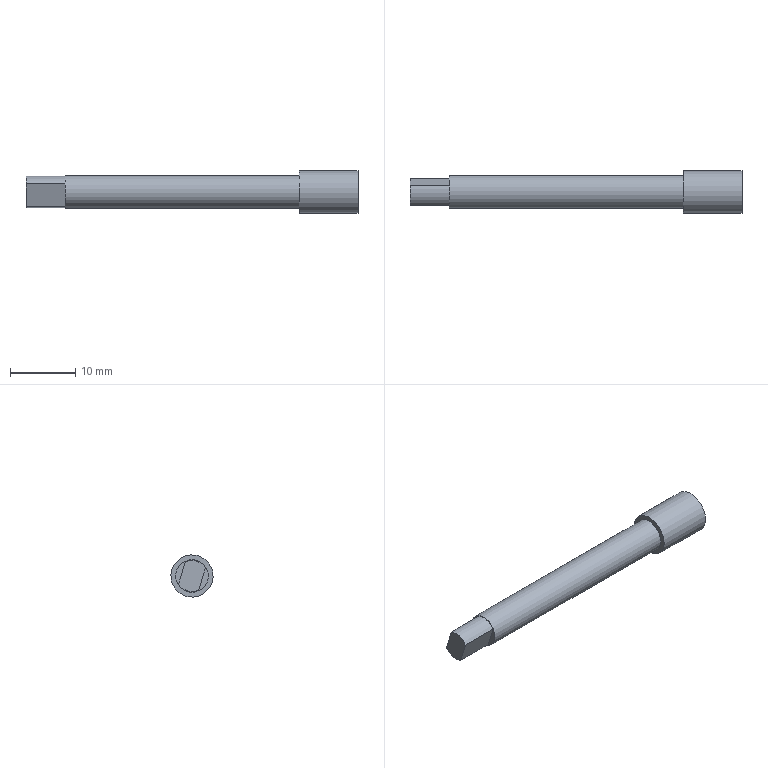Part | STEP file | Dodanie-wyci_gni_cie4_1 | 1 solid | 15 faces | box 51 x 6.5 x 6.5 mm | volume 982.022 mm3 | plane 9 | cylinder 6 | commonest cylinder face diameters 5 x3 4.8 x2 6.5 x1
STEP:
#1=CARTESIAN_POINT('',(0.,0.,0.));
#2=DIRECTION('',(0.,0.,1.));
#3=DIRECTION('',(1.,0.,0.));
#4=AXIS2_PLACEMENT_3D('',#1,#2,#3);
#5=CARTESIAN_POINT('',(-60.496,90.397,-74.615));
#6=VERTEX_POINT('',#5);
#7=CARTESIAN_POINT('',(-96.496,90.397,-74.615));
#8=VERTEX_POINT('',#7);
#9=CARTESIAN_POINT('',(-60.496,90.397,-74.615));
#10=DIRECTION('',(-1.,0.,0.));
#11=VECTOR('',#10,1.);
#12=LINE('',#9,#11);
#13=CARTESIAN_POINT('',(-96.496,88.009,-75.356));
#14=DIRECTION('',(1.,0.,0.));
#15=DIRECTION('',(0.,0.9551,0.2962));
#16=AXIS2_PLACEMENT_3D('',#13,#14,#15);
#17=CYLINDRICAL_SURFACE('',#16,2.5);
#18=CARTESIAN_POINT('',(0.,36.));
#19=DIRECTION('',(0.,-1.));
#20=VECTOR('',#19,1.);
#21=LINE('',#18,#20);
#22=(GEOMETRIC_REPRESENTATION_CONTEXT(2)PARAMETRIC_REPRESENTATION_CONTEXT()REPRESENTATION_CONTEXT('',''));
#23=DEFINITIONAL_REPRESENTATION('',(#21),#22);
#24=PCURVE('',#17,#23);
#25=CARTESIAN_POINT('',(6.283,36.));
#26=DIRECTION('',(0.,-1.));
#27=VECTOR('',#26,1.);
#28=LINE('',#25,#27);
#29=(GEOMETRIC_REPRESENTATION_CONTEXT(2)PARAMETRIC_REPRESENTATION_CONTEXT()REPRESENTATION_CONTEXT('',''));
#30=DEFINITIONAL_REPRESENTATION('',(#28),#29);
#31=PCURVE('',#17,#30);
#32=SEAM_CURVE('',#12,(#24,#31),.PCURVE_S1.);
#33=EDGE_CURVE('',#6,#8,#32,.T.);
#34=ORIENTED_EDGE('',*,*,#33,.T.);
#35=CARTESIAN_POINT('',(-96.496,88.009,-75.356));
#36=DIRECTION('',(1.,0.,0.));
#37=DIRECTION('',(0.,0.9551,0.2962));
#38=AXIS2_PLACEMENT_3D('',#35,#36,#37);
#39=CIRCLE('',#38,2.5);
#40=CARTESIAN_POINT('',(0.,0.));
#41=DIRECTION('',(1.,0.));
#42=VECTOR('',#41,1.);
#43=LINE('',#40,#42);
#44=(GEOMETRIC_REPRESENTATION_CONTEXT(2)PARAMETRIC_REPRESENTATION_CONTEXT()REPRESENTATION_CONTEXT('',''));
#45=DEFINITIONAL_REPRESENTATION('',(#43),#44);
#46=PCURVE('',#17,#45);
#47=CARTESIAN_POINT('',(-96.496,88.009,-75.356));
#48=DIRECTION('',(-1.,0.,0.));
#49=DIRECTION('',(0.,-0.9551,-0.2962));
#50=AXIS2_PLACEMENT_3D('',#47,#48,#49);
#51=PLANE('',#50);
#52=CARTESIAN_POINT('',(-2.5,0.));
#53=CARTESIAN_POINT('',(-2.5,4.33));
#54=CARTESIAN_POINT('',(1.25,2.165));
#55=CARTESIAN_POINT('',(5.,0.));
#56=CARTESIAN_POINT('',(1.25,-2.165));
#57=CARTESIAN_POINT('',(-2.5,-4.33));
#58=CARTESIAN_POINT('',(-2.5,0.));
#59=(BOUNDED_CURVE()B_SPLINE_CURVE(2,(#52,#53,#54,#55,#56,#57,#58),.UNSPECIFIED.,.T.,.F.)B_SPLINE_CURVE_WITH_KNOTS((1,2,2,2,2,1),(-2.094,0.,2.094,4.189,6.283,8.378),.UNSPECIFIED.)CURVE()GEOMETRIC_REPRESENTATION_ITEM()RATIONAL_B_SPLINE_CURVE((1.,0.5,1.,0.5,1.,0.5,1.))REPRESENTATION_ITEM(''));
#60=(GEOMETRIC_REPRESENTATION_CONTEXT(2)PARAMETRIC_REPRESENTATION_CONTEXT()REPRESENTATION_CONTEXT('',''));
#61=DEFINITIONAL_REPRESENTATION('',(#59),#60);
#62=PCURVE('',#51,#61);
#63=SURFACE_CURVE('',#39,(#46,#62),.PCURVE_S1.);
#64=EDGE_CURVE('',#8,#8,#63,.T.);
#65=ORIENTED_EDGE('',*,*,#64,.T.);
#66=ORIENTED_EDGE('',*,*,#33,.F.);
#67=CARTESIAN_POINT('',(-60.496,88.009,-75.356));
#68=DIRECTION('',(-1.,0.,0.));
#69=DIRECTION('',(0.,0.9551,0.2962));
#70=AXIS2_PLACEMENT_3D('',#67,#68,#69);
#71=CIRCLE('',#70,2.5);
#72=CARTESIAN_POINT('',(6.283,36.));
#73=DIRECTION('',(-1.,0.));
#74=VECTOR('',#73,1.);
#75=LINE('',#72,#74);
#76=(GEOMETRIC_REPRESENTATION_CONTEXT(2)PARAMETRIC_REPRESENTATION_CONTEXT()REPRESENTATION_CONTEXT('',''));
#77=DEFINITIONAL_REPRESENTATION('',(#75),#76);
#78=PCURVE('',#17,#77);
#79=CARTESIAN_POINT('',(-60.496,88.009,-75.356));
#80=DIRECTION('',(-1.,0.,0.));
#81=DIRECTION('',(0.,-0.9551,-0.2962));
#82=AXIS2_PLACEMENT_3D('',#79,#80,#81);
#83=PLANE('',#82);
#84=CARTESIAN_POINT('',(0.,0.));
#85=DIRECTION('',(-1.,0.));
#86=AXIS2_PLACEMENT_2D('',#84,#85);
#87=CIRCLE('',#86,2.5);
#88=(GEOMETRIC_REPRESENTATION_CONTEXT(2)PARAMETRIC_REPRESENTATION_CONTEXT()REPRESENTATION_CONTEXT('',''));
#89=DEFINITIONAL_REPRESENTATION('',(#87),#88);
#90=PCURVE('',#83,#89);
#91=SURFACE_CURVE('',#71,(#78,#90),.PCURVE_S1.);
#92=EDGE_CURVE('',#6,#6,#91,.T.);
#93=ORIENTED_EDGE('',*,*,#92,.T.);
#94=EDGE_LOOP('',(#34,#65,#66,#93));
#95=FACE_BOUND('',#94,.T.);
#96=ADVANCED_FACE('',(#95),#17,.T.);
#97=CARTESIAN_POINT('',(-51.496,91.113,-74.393));
#98=VERTEX_POINT('',#97);
#99=CARTESIAN_POINT('',(-60.496,91.113,-74.393));
#100=VERTEX_POINT('',#99);
#101=CARTESIAN_POINT('',(-51.496,91.113,-74.393));
#102=DIRECTION('',(-1.,0.,0.));
#103=VECTOR('',#102,1.);
#104=LINE('',#101,#103);
#105=CARTESIAN_POINT('',(-60.496,88.009,-75.356));
#106=DIRECTION('',(1.,0.,0.));
#107=DIRECTION('',(0.,0.9551,0.2962));
#108=AXIS2_PLACEMENT_3D('',#105,#106,#107);
#109=CYLINDRICAL_SURFACE('',#108,3.25);
#110=CARTESIAN_POINT('',(0.,9.));
#111=DIRECTION('',(0.,-1.));
#112=VECTOR('',#111,1.);
#113=LINE('',#110,#112);
#114=(GEOMETRIC_REPRESENTATION_CONTEXT(2)PARAMETRIC_REPRESENTATION_CONTEXT()REPRESENTATION_CONTEXT('',''));
#115=DEFINITIONAL_REPRESENTATION('',(#113),#114);
#116=PCURVE('',#109,#115);
#117=CARTESIAN_POINT('',(6.283,9.));
#118=DIRECTION('',(0.,-1.));
#119=VECTOR('',#118,1.);
#120=LINE('',#117,#119);
#121=(GEOMETRIC_REPRESENTATION_CONTEXT(2)PARAMETRIC_REPRESENTATION_CONTEXT()REPRESENTATION_CONTEXT('',''));
#122=DEFINITIONAL_REPRESENTATION('',(#120),#121);
#123=PCURVE('',#109,#122);
#124=SEAM_CURVE('',#104,(#116,#123),.PCURVE_S1.);
#125=EDGE_CURVE('',#98,#100,#124,.T.);
#126=ORIENTED_EDGE('',*,*,#125,.T.);
#127=CARTESIAN_POINT('',(-60.496,88.009,-75.356));
#128=DIRECTION('',(-1.,0.,0.));
#129=DIRECTION('',(0.,0.9551,0.2962));
#130=AXIS2_PLACEMENT_3D('',#127,#128,#129);
#131=CIRCLE('',#130,3.25);
#132=CARTESIAN_POINT('',(6.283,0.));
#133=DIRECTION('',(-1.,0.));
#134=VECTOR('',#133,1.);
#135=LINE('',#132,#134);
#136=(GEOMETRIC_REPRESENTATION_CONTEXT(2)PARAMETRIC_REPRESENTATION_CONTEXT()REPRESENTATION_CONTEXT('',''));
#137=DEFINITIONAL_REPRESENTATION('',(#135),#136);
#138=PCURVE('',#109,#137);
#139=CARTESIAN_POINT('',(0.,0.));
#140=DIRECTION('',(-1.,0.));
#141=AXIS2_PLACEMENT_2D('',#139,#140);
#142=CIRCLE('',#141,3.25);
#143=(GEOMETRIC_REPRESENTATION_CONTEXT(2)PARAMETRIC_REPRESENTATION_CONTEXT()REPRESENTATION_CONTEXT('',''));
#144=DEFINITIONAL_REPRESENTATION('',(#142),#143);
#145=PCURVE('',#83,#144);
#146=SURFACE_CURVE('',#131,(#138,#145),.PCURVE_S1.);
#147=EDGE_CURVE('',#100,#100,#146,.T.);
#148=ORIENTED_EDGE('',*,*,#147,.F.);
#149=ORIENTED_EDGE('',*,*,#125,.F.);
#150=CARTESIAN_POINT('',(-51.496,88.009,-75.356));
#151=DIRECTION('',(-1.,0.,0.));
#152=DIRECTION('',(0.,0.9551,0.2962));
#153=AXIS2_PLACEMENT_3D('',#150,#151,#152);
#154=CIRCLE('',#153,3.25);
#155=CARTESIAN_POINT('',(6.283,9.));
#156=DIRECTION('',(-1.,0.));
#157=VECTOR('',#156,1.);
#158=LINE('',#155,#157);
#159=(GEOMETRIC_REPRESENTATION_CONTEXT(2)PARAMETRIC_REPRESENTATION_CONTEXT()REPRESENTATION_CONTEXT('',''));
#160=DEFINITIONAL_REPRESENTATION('',(#158),#159);
#161=PCURVE('',#109,#160);
#162=CARTESIAN_POINT('',(-51.496,88.009,-75.356));
#163=DIRECTION('',(-1.,0.,0.));
#164=DIRECTION('',(0.,-0.9551,-0.2962));
#165=AXIS2_PLACEMENT_3D('',#162,#163,#164);
#166=PLANE('',#165);
#167=CARTESIAN_POINT('',(0.,0.));
#168=DIRECTION('',(-1.,0.));
#169=AXIS2_PLACEMENT_2D('',#167,#168);
#170=CIRCLE('',#169,3.25);
#171=(GEOMETRIC_REPRESENTATION_CONTEXT(2)PARAMETRIC_REPRESENTATION_CONTEXT()REPRESENTATION_CONTEXT('',''));
#172=DEFINITIONAL_REPRESENTATION('',(#170),#171);
#173=PCURVE('',#166,#172);
#174=SURFACE_CURVE('',#154,(#161,#173),.PCURVE_S1.);
#175=EDGE_CURVE('',#98,#98,#174,.T.);
#176=ORIENTED_EDGE('',*,*,#175,.T.);
#177=EDGE_LOOP('',(#126,#148,#149,#176));
#178=FACE_BOUND('',#177,.T.);
#179=ADVANCED_FACE('',(#178),#109,.T.);
#180=ORIENTED_EDGE('',*,*,#92,.F.);
#181=EDGE_LOOP('',(#180));
#182=FACE_BOUND('',#181,.T.);
#183=ORIENTED_EDGE('',*,*,#147,.T.);
#184=EDGE_LOOP('',(#183));
#185=FACE_BOUND('',#184,.T.);
#186=ADVANCED_FACE('',(#182,#185),#83,.T.);
#187=CARTESIAN_POINT('',(-96.496,89.008,-73.173));
#188=VERTEX_POINT('',#187);
#189=CARTESIAN_POINT('',(-96.496,85.951,-74.121));
#190=VERTEX_POINT('',#189);
#191=CARTESIAN_POINT('',(-96.496,88.009,-75.356));
#192=DIRECTION('',(1.,0.,0.));
#193=DIRECTION('',(0.,0.9551,0.2962));
#194=AXIS2_PLACEMENT_3D('',#191,#192,#193);
#195=CIRCLE('',#194,2.4);
#196=CARTESIAN_POINT('',(-2.4,0.));
#197=CARTESIAN_POINT('',(-2.4,4.157));
#198=CARTESIAN_POINT('',(1.2,2.078));
#199=CARTESIAN_POINT('',(4.8,0.));
#200=CARTESIAN_POINT('',(1.2,-2.078));
#201=CARTESIAN_POINT('',(-2.4,-4.157));
#202=CARTESIAN_POINT('',(-2.4,0.));
#203=(BOUNDED_CURVE()B_SPLINE_CURVE(2,(#196,#197,#198,#199,#200,#201,#202),.UNSPECIFIED.,.T.,.F.)B_SPLINE_CURVE_WITH_KNOTS((1,2,2,2,2,1),(-2.094,0.,2.094,4.189,6.283,8.378),.UNSPECIFIED.)CURVE()GEOMETRIC_REPRESENTATION_ITEM()RATIONAL_B_SPLINE_CURVE((1.,0.5,1.,0.5,1.,0.5,1.))REPRESENTATION_ITEM(''));
#204=(GEOMETRIC_REPRESENTATION_CONTEXT(2)PARAMETRIC_REPRESENTATION_CONTEXT()REPRESENTATION_CONTEXT('',''));
#205=DEFINITIONAL_REPRESENTATION('',(#203),#204);
#206=PCURVE('',#51,#205);
#207=CARTESIAN_POINT('',(-102.496,88.009,-75.356));
#208=DIRECTION('',(1.,0.,0.));
#209=DIRECTION('',(0.,0.9551,0.2962));
#210=AXIS2_PLACEMENT_3D('',#207,#208,#209);
#211=CYLINDRICAL_SURFACE('',#210,2.4);
#212=CARTESIAN_POINT('',(0.,6.));
#213=DIRECTION('',(1.,0.));
#214=VECTOR('',#213,1.);
#215=LINE('',#212,#214);
#216=(GEOMETRIC_REPRESENTATION_CONTEXT(2)PARAMETRIC_REPRESENTATION_CONTEXT()REPRESENTATION_CONTEXT('',''));
#217=DEFINITIONAL_REPRESENTATION('',(#215),#216);
#218=PCURVE('',#211,#217);
#219=SURFACE_CURVE('',#195,(#206,#218),.PCURVE_S1.);
#220=EDGE_CURVE('',#188,#190,#219,.T.);
#221=ORIENTED_EDGE('',*,*,#220,.T.);
#222=CARTESIAN_POINT('',(-96.496,87.011,-77.538));
#223=VERTEX_POINT('',#222);
#224=CARTESIAN_POINT('',(-96.496,85.951,-74.121));
#225=DIRECTION('',(0.,0.2962,-0.9551));
#226=VECTOR('',#225,1.);
#227=LINE('',#224,#226);
#228=CARTESIAN_POINT('',(1.6,1.789));
#229=DIRECTION('',(0.,-1.));
#230=VECTOR('',#229,1.);
#231=LINE('',#228,#230);
#232=(GEOMETRIC_REPRESENTATION_CONTEXT(2)PARAMETRIC_REPRESENTATION_CONTEXT()REPRESENTATION_CONTEXT('',''));
#233=DEFINITIONAL_REPRESENTATION('',(#231),#232);
#234=PCURVE('',#51,#233);
#235=CARTESIAN_POINT('',(-99.496,86.481,-75.83));
#236=DIRECTION('',(0.,0.9551,0.2962));
#237=DIRECTION('',(-1.,0.,0.));
#238=AXIS2_PLACEMENT_3D('',#235,#236,#237);
#239=PLANE('',#238);
#240=CARTESIAN_POINT('',(-3.,1.789));
#241=DIRECTION('',(0.,-1.));
#242=VECTOR('',#241,1.);
#243=LINE('',#240,#242);
#244=(GEOMETRIC_REPRESENTATION_CONTEXT(2)PARAMETRIC_REPRESENTATION_CONTEXT()REPRESENTATION_CONTEXT('',''));
#245=DEFINITIONAL_REPRESENTATION('',(#243),#244);
#246=PCURVE('',#239,#245);
#247=SURFACE_CURVE('',#227,(#234,#246),.PCURVE_S1.);
#248=EDGE_CURVE('',#190,#223,#247,.T.);
#249=ORIENTED_EDGE('',*,*,#248,.T.);
#250=CARTESIAN_POINT('',(-96.496,90.067,-76.59));
#251=VERTEX_POINT('',#250);
#252=CARTESIAN_POINT('',(-96.496,88.009,-75.356));
#253=DIRECTION('',(1.,0.,0.));
#254=DIRECTION('',(0.,0.9551,0.2962));
#255=AXIS2_PLACEMENT_3D('',#252,#253,#254);
#256=CIRCLE('',#255,2.4);
#257=CARTESIAN_POINT('',(-2.4,0.));
#258=CARTESIAN_POINT('',(-2.4,4.157));
#259=CARTESIAN_POINT('',(1.2,2.078));
#260=CARTESIAN_POINT('',(4.8,0.));
#261=CARTESIAN_POINT('',(1.2,-2.078));
#262=CARTESIAN_POINT('',(-2.4,-4.157));
#263=CARTESIAN_POINT('',(-2.4,0.));
#264=(BOUNDED_CURVE()B_SPLINE_CURVE(2,(#257,#258,#259,#260,#261,#262,#263),.UNSPECIFIED.,.T.,.F.)B_SPLINE_CURVE_WITH_KNOTS((1,2,2,2,2,1),(-2.094,0.,2.094,4.189,6.283,8.378),.UNSPECIFIED.)CURVE()GEOMETRIC_REPRESENTATION_ITEM()RATIONAL_B_SPLINE_CURVE((1.,0.5,1.,0.5,1.,0.5,1.))REPRESENTATION_ITEM(''));
#265=(GEOMETRIC_REPRESENTATION_CONTEXT(2)PARAMETRIC_REPRESENTATION_CONTEXT()REPRESENTATION_CONTEXT('',''));
#266=DEFINITIONAL_REPRESENTATION('',(#264),#265);
#267=PCURVE('',#51,#266);
#268=CARTESIAN_POINT('',(-102.496,88.009,-75.356));
#269=DIRECTION('',(1.,0.,0.));
#270=DIRECTION('',(0.,0.9551,0.2962));
#271=AXIS2_PLACEMENT_3D('',#268,#269,#270);
#272=CYLINDRICAL_SURFACE('',#271,2.4);
#273=CARTESIAN_POINT('',(0.,6.));
#274=DIRECTION('',(1.,0.));
#275=VECTOR('',#274,1.);
#276=LINE('',#273,#275);
#277=(GEOMETRIC_REPRESENTATION_CONTEXT(2)PARAMETRIC_REPRESENTATION_CONTEXT()REPRESENTATION_CONTEXT('',''));
#278=DEFINITIONAL_REPRESENTATION('',(#276),#277);
#279=PCURVE('',#272,#278);
#280=SURFACE_CURVE('',#256,(#267,#279),.PCURVE_S1.);
#281=EDGE_CURVE('',#223,#251,#280,.T.);
#282=ORIENTED_EDGE('',*,*,#281,.T.);
#283=CARTESIAN_POINT('',(-96.496,90.067,-76.59));
#284=DIRECTION('',(0.,-0.2962,0.9551));
#285=VECTOR('',#284,1.);
#286=LINE('',#283,#285);
#287=CARTESIAN_POINT('',(-1.6,-1.789));
#288=DIRECTION('',(0.,1.));
#289=VECTOR('',#288,1.);
#290=LINE('',#287,#289);
#291=(GEOMETRIC_REPRESENTATION_CONTEXT(2)PARAMETRIC_REPRESENTATION_CONTEXT()REPRESENTATION_CONTEXT('',''));
#292=DEFINITIONAL_REPRESENTATION('',(#290),#291);
#293=PCURVE('',#51,#292);
#294=CARTESIAN_POINT('',(-99.496,89.537,-74.882));
#295=DIRECTION('',(0.,-0.9551,-0.2962));
#296=DIRECTION('',(1.,0.,0.));
#297=AXIS2_PLACEMENT_3D('',#294,#295,#296);
#298=PLANE('',#297);
#299=CARTESIAN_POINT('',(3.,-1.789));
#300=DIRECTION('',(0.,1.));
#301=VECTOR('',#300,1.);
#302=LINE('',#299,#301);
#303=(GEOMETRIC_REPRESENTATION_CONTEXT(2)PARAMETRIC_REPRESENTATION_CONTEXT()REPRESENTATION_CONTEXT('',''));
#304=DEFINITIONAL_REPRESENTATION('',(#302),#303);
#305=PCURVE('',#298,#304);
#306=SURFACE_CURVE('',#286,(#293,#305),.PCURVE_S1.);
#307=EDGE_CURVE('',#251,#188,#306,.T.);
#308=ORIENTED_EDGE('',*,*,#307,.T.);
#309=EDGE_LOOP('',(#221,#249,#282,#308));
#310=FACE_BOUND('',#309,.T.);
#311=ORIENTED_EDGE('',*,*,#64,.F.);
#312=EDGE_LOOP('',(#311));
#313=FACE_BOUND('',#312,.T.);
#314=ADVANCED_FACE('',(#310,#313),#51,.T.);
#315=CARTESIAN_POINT('',(-102.496,85.951,-74.121));
#316=VERTEX_POINT('',#315);
#317=CARTESIAN_POINT('',(-102.496,85.951,-74.121));
#318=DIRECTION('',(1.,0.,0.));
#319=VECTOR('',#318,1.);
#320=LINE('',#317,#319);
#321=CARTESIAN_POINT('',(3.,1.789));
#322=DIRECTION('',(-1.,0.));
#323=VECTOR('',#322,1.);
#324=LINE('',#321,#323);
#325=(GEOMETRIC_REPRESENTATION_CONTEXT(2)PARAMETRIC_REPRESENTATION_CONTEXT()REPRESENTATION_CONTEXT('',''));
#326=DEFINITIONAL_REPRESENTATION('',(#324),#325);
#327=PCURVE('',#239,#326);
#328=CARTESIAN_POINT('',(2.301,0.));
#329=DIRECTION('',(0.,1.));
#330=VECTOR('',#329,1.);
#331=LINE('',#328,#330);
#332=(GEOMETRIC_REPRESENTATION_CONTEXT(2)PARAMETRIC_REPRESENTATION_CONTEXT()REPRESENTATION_CONTEXT('',''));
#333=DEFINITIONAL_REPRESENTATION('',(#331),#332);
#334=PCURVE('',#211,#333);
#335=SURFACE_CURVE('',#320,(#327,#334),.PCURVE_S1.);
#336=EDGE_CURVE('',#316,#190,#335,.T.);
#337=ORIENTED_EDGE('',*,*,#336,.F.);
#338=CARTESIAN_POINT('',(-102.496,87.011,-77.538));
#339=VERTEX_POINT('',#338);
#340=CARTESIAN_POINT('',(-102.496,87.011,-77.538));
#341=DIRECTION('',(0.,-0.2962,0.9551));
#342=VECTOR('',#341,1.);
#343=LINE('',#340,#342);
#344=CARTESIAN_POINT('',(3.,-1.789));
#345=DIRECTION('',(0.,1.));
#346=VECTOR('',#345,1.);
#347=LINE('',#344,#346);
#348=(GEOMETRIC_REPRESENTATION_CONTEXT(2)PARAMETRIC_REPRESENTATION_CONTEXT()REPRESENTATION_CONTEXT('',''));
#349=DEFINITIONAL_REPRESENTATION('',(#347),#348);
#350=PCURVE('',#239,#349);
#351=CARTESIAN_POINT('',(-102.496,88.009,-75.356));
#352=DIRECTION('',(-1.,0.,0.));
#353=DIRECTION('',(0.,-0.9551,-0.2962));
#354=AXIS2_PLACEMENT_3D('',#351,#352,#353);
#355=PLANE('',#354);
#356=CARTESIAN_POINT('',(1.6,-1.789));
#357=DIRECTION('',(0.,1.));
#358=VECTOR('',#357,1.);
#359=LINE('',#356,#358);
#360=(GEOMETRIC_REPRESENTATION_CONTEXT(2)PARAMETRIC_REPRESENTATION_CONTEXT()REPRESENTATION_CONTEXT('',''));
#361=DEFINITIONAL_REPRESENTATION('',(#359),#360);
#362=PCURVE('',#355,#361);
#363=SURFACE_CURVE('',#343,(#350,#362),.PCURVE_S1.);
#364=EDGE_CURVE('',#339,#316,#363,.T.);
#365=ORIENTED_EDGE('',*,*,#364,.F.);
#366=CARTESIAN_POINT('',(-96.496,87.011,-77.538));
#367=DIRECTION('',(-1.,0.,0.));
#368=VECTOR('',#367,1.);
#369=LINE('',#366,#368);
#370=CARTESIAN_POINT('',(-3.,-1.789));
#371=DIRECTION('',(1.,0.));
#372=VECTOR('',#371,1.);
#373=LINE('',#370,#372);
#374=(GEOMETRIC_REPRESENTATION_CONTEXT(2)PARAMETRIC_REPRESENTATION_CONTEXT()REPRESENTATION_CONTEXT('',''));
#375=DEFINITIONAL_REPRESENTATION('',(#373),#374);
#376=PCURVE('',#239,#375);
#377=CARTESIAN_POINT('',(3.983,6.));
#378=DIRECTION('',(0.,-1.));
#379=VECTOR('',#378,1.);
#380=LINE('',#377,#379);
#381=(GEOMETRIC_REPRESENTATION_CONTEXT(2)PARAMETRIC_REPRESENTATION_CONTEXT()REPRESENTATION_CONTEXT('',''));
#382=DEFINITIONAL_REPRESENTATION('',(#380),#381);
#383=PCURVE('',#272,#382);
#384=SURFACE_CURVE('',#369,(#376,#383),.PCURVE_S1.);
#385=EDGE_CURVE('',#223,#339,#384,.T.);
#386=ORIENTED_EDGE('',*,*,#385,.F.);
#387=ORIENTED_EDGE('',*,*,#248,.F.);
#388=EDGE_LOOP('',(#337,#365,#386,#387));
#389=FACE_BOUND('',#388,.T.);
#390=ADVANCED_FACE('',(#389),#239,.F.);
#391=CARTESIAN_POINT('',(-102.496,89.008,-73.173));
#392=VERTEX_POINT('',#391);
#393=CARTESIAN_POINT('',(-102.496,88.009,-75.356));
#394=DIRECTION('',(1.,0.,0.));
#395=DIRECTION('',(0.,0.9551,0.2962));
#396=AXIS2_PLACEMENT_3D('',#393,#394,#395);
#397=CIRCLE('',#396,2.4);
#398=CARTESIAN_POINT('',(0.,0.));
#399=DIRECTION('',(1.,0.));
#400=VECTOR('',#399,1.);
#401=LINE('',#398,#400);
#402=(GEOMETRIC_REPRESENTATION_CONTEXT(2)PARAMETRIC_REPRESENTATION_CONTEXT()REPRESENTATION_CONTEXT('',''));
#403=DEFINITIONAL_REPRESENTATION('',(#401),#402);
#404=PCURVE('',#211,#403);
#405=CARTESIAN_POINT('',(-2.4,0.));
#406=CARTESIAN_POINT('',(-2.4,4.157));
#407=CARTESIAN_POINT('',(1.2,2.078));
#408=CARTESIAN_POINT('',(4.8,0.));
#409=CARTESIAN_POINT('',(1.2,-2.078));
#410=CARTESIAN_POINT('',(-2.4,-4.157));
#411=CARTESIAN_POINT('',(-2.4,0.));
#412=(BOUNDED_CURVE()B_SPLINE_CURVE(2,(#405,#406,#407,#408,#409,#410,#411),.UNSPECIFIED.,.T.,.F.)B_SPLINE_CURVE_WITH_KNOTS((1,2,2,2,2,1),(-2.094,0.,2.094,4.189,6.283,8.378),.UNSPECIFIED.)CURVE()GEOMETRIC_REPRESENTATION_ITEM()RATIONAL_B_SPLINE_CURVE((1.,0.5,1.,0.5,1.,0.5,1.))REPRESENTATION_ITEM(''));
#413=(GEOMETRIC_REPRESENTATION_CONTEXT(2)PARAMETRIC_REPRESENTATION_CONTEXT()REPRESENTATION_CONTEXT('',''));
#414=DEFINITIONAL_REPRESENTATION('',(#412),#413);
#415=PCURVE('',#355,#414);
#416=SURFACE_CURVE('',#397,(#404,#415),.PCURVE_S1.);
#417=EDGE_CURVE('',#392,#316,#416,.T.);
#418=ORIENTED_EDGE('',*,*,#417,.T.);
#419=ORIENTED_EDGE('',*,*,#336,.T.);
#420=ORIENTED_EDGE('',*,*,#220,.F.);
#421=CARTESIAN_POINT('',(-96.496,89.008,-73.173));
#422=DIRECTION('',(-1.,0.,0.));
#423=VECTOR('',#422,1.);
#424=LINE('',#421,#423);
#425=CARTESIAN_POINT('',(0.8411,6.));
#426=DIRECTION('',(0.,-1.));
#427=VECTOR('',#426,1.);
#428=LINE('',#425,#427);
#429=(GEOMETRIC_REPRESENTATION_CONTEXT(2)PARAMETRIC_REPRESENTATION_CONTEXT()REPRESENTATION_CONTEXT('',''));
#430=DEFINITIONAL_REPRESENTATION('',(#428),#429);
#431=PCURVE('',#211,#430);
#432=CARTESIAN_POINT('',(3.,1.789));
#433=DIRECTION('',(-1.,0.));
#434=VECTOR('',#433,1.);
#435=LINE('',#432,#434);
#436=(GEOMETRIC_REPRESENTATION_CONTEXT(2)PARAMETRIC_REPRESENTATION_CONTEXT()REPRESENTATION_CONTEXT('',''));
#437=DEFINITIONAL_REPRESENTATION('',(#435),#436);
#438=PCURVE('',#298,#437);
#439=SURFACE_CURVE('',#424,(#431,#438),.PCURVE_S1.);
#440=EDGE_CURVE('',#188,#392,#439,.T.);
#441=ORIENTED_EDGE('',*,*,#440,.T.);
#442=EDGE_LOOP('',(#418,#419,#420,#441));
#443=FACE_BOUND('',#442,.T.);
#444=ADVANCED_FACE('',(#443),#211,.T.);
#445=CARTESIAN_POINT('',(-102.496,90.067,-76.59));
#446=VERTEX_POINT('',#445);
#447=CARTESIAN_POINT('',(-102.496,90.067,-76.59));
#448=DIRECTION('',(1.,0.,0.));
#449=VECTOR('',#448,1.);
#450=LINE('',#447,#449);
#451=CARTESIAN_POINT('',(-3.,-1.789));
#452=DIRECTION('',(1.,0.));
#453=VECTOR('',#452,1.);
#454=LINE('',#451,#453);
#455=(GEOMETRIC_REPRESENTATION_CONTEXT(2)PARAMETRIC_REPRESENTATION_CONTEXT()REPRESENTATION_CONTEXT('',''));
#456=DEFINITIONAL_REPRESENTATION('',(#454),#455);
#457=PCURVE('',#298,#456);
#458=CARTESIAN_POINT('',(5.442,0.));
#459=DIRECTION('',(0.,1.));
#460=VECTOR('',#459,1.);
#461=LINE('',#458,#460);
#462=(GEOMETRIC_REPRESENTATION_CONTEXT(2)PARAMETRIC_REPRESENTATION_CONTEXT()REPRESENTATION_CONTEXT('',''));
#463=DEFINITIONAL_REPRESENTATION('',(#461),#462);
#464=PCURVE('',#272,#463);
#465=SURFACE_CURVE('',#450,(#457,#464),.PCURVE_S1.);
#466=EDGE_CURVE('',#446,#251,#465,.T.);
#467=ORIENTED_EDGE('',*,*,#466,.F.);
#468=CARTESIAN_POINT('',(-102.496,89.008,-73.173));
#469=DIRECTION('',(0.,0.2962,-0.9551));
#470=VECTOR('',#469,1.);
#471=LINE('',#468,#470);
#472=CARTESIAN_POINT('',(-3.,1.789));
#473=DIRECTION('',(0.,-1.));
#474=VECTOR('',#473,1.);
#475=LINE('',#472,#474);
#476=(GEOMETRIC_REPRESENTATION_CONTEXT(2)PARAMETRIC_REPRESENTATION_CONTEXT()REPRESENTATION_CONTEXT('',''));
#477=DEFINITIONAL_REPRESENTATION('',(#475),#476);
#478=PCURVE('',#298,#477);
#479=CARTESIAN_POINT('',(-1.6,1.789));
#480=DIRECTION('',(0.,-1.));
#481=VECTOR('',#480,1.);
#482=LINE('',#479,#481);
#483=(GEOMETRIC_REPRESENTATION_CONTEXT(2)PARAMETRIC_REPRESENTATION_CONTEXT()REPRESENTATION_CONTEXT('',''));
#484=DEFINITIONAL_REPRESENTATION('',(#482),#483);
#485=PCURVE('',#355,#484);
#486=SURFACE_CURVE('',#471,(#478,#485),.PCURVE_S1.);
#487=EDGE_CURVE('',#392,#446,#486,.T.);
#488=ORIENTED_EDGE('',*,*,#487,.F.);
#489=ORIENTED_EDGE('',*,*,#440,.F.);
#490=ORIENTED_EDGE('',*,*,#307,.F.);
#491=EDGE_LOOP('',(#467,#488,#489,#490));
#492=FACE_BOUND('',#491,.T.);
#493=ADVANCED_FACE('',(#492),#298,.F.);
#494=CARTESIAN_POINT('',(-102.496,88.009,-75.356));
#495=DIRECTION('',(1.,0.,0.));
#496=DIRECTION('',(0.,0.9551,0.2962));
#497=AXIS2_PLACEMENT_3D('',#494,#495,#496);
#498=CIRCLE('',#497,2.4);
#499=CARTESIAN_POINT('',(0.,0.));
#500=DIRECTION('',(1.,0.));
#501=VECTOR('',#500,1.);
#502=LINE('',#499,#501);
#503=(GEOMETRIC_REPRESENTATION_CONTEXT(2)PARAMETRIC_REPRESENTATION_CONTEXT()REPRESENTATION_CONTEXT('',''));
#504=DEFINITIONAL_REPRESENTATION('',(#502),#503);
#505=PCURVE('',#272,#504);
#506=CARTESIAN_POINT('',(-2.4,0.));
#507=CARTESIAN_POINT('',(-2.4,4.157));
#508=CARTESIAN_POINT('',(1.2,2.078));
#509=CARTESIAN_POINT('',(4.8,0.));
#510=CARTESIAN_POINT('',(1.2,-2.078));
#511=CARTESIAN_POINT('',(-2.4,-4.157));
#512=CARTESIAN_POINT('',(-2.4,0.));
#513=(BOUNDED_CURVE()B_SPLINE_CURVE(2,(#506,#507,#508,#509,#510,#511,#512),.UNSPECIFIED.,.T.,.F.)B_SPLINE_CURVE_WITH_KNOTS((1,2,2,2,2,1),(-2.094,0.,2.094,4.189,6.283,8.378),.UNSPECIFIED.)CURVE()GEOMETRIC_REPRESENTATION_ITEM()RATIONAL_B_SPLINE_CURVE((1.,0.5,1.,0.5,1.,0.5,1.))REPRESENTATION_ITEM(''));
#514=(GEOMETRIC_REPRESENTATION_CONTEXT(2)PARAMETRIC_REPRESENTATION_CONTEXT()REPRESENTATION_CONTEXT('',''));
#515=DEFINITIONAL_REPRESENTATION('',(#513),#514);
#516=PCURVE('',#355,#515);
#517=SURFACE_CURVE('',#498,(#505,#516),.PCURVE_S1.);
#518=EDGE_CURVE('',#339,#446,#517,.T.);
#519=ORIENTED_EDGE('',*,*,#518,.T.);
#520=ORIENTED_EDGE('',*,*,#466,.T.);
#521=ORIENTED_EDGE('',*,*,#281,.F.);
#522=ORIENTED_EDGE('',*,*,#385,.T.);
#523=EDGE_LOOP('',(#519,#520,#521,#522));
#524=FACE_BOUND('',#523,.T.);
#525=ADVANCED_FACE('',(#524),#272,.T.);
#526=CARTESIAN_POINT('',(-51.496,86.031,-73.828));
#527=VERTEX_POINT('',#526);
#528=CARTESIAN_POINT('',(-51.496,87.243,-77.735));
#529=VERTEX_POINT('',#528);
#530=CARTESIAN_POINT('',(-51.496,86.031,-73.828));
#531=DIRECTION('',(0.,0.2962,-0.9551));
#532=VECTOR('',#531,1.);
#533=LINE('',#530,#532);
#534=CARTESIAN_POINT('',(1.437,2.046));
#535=DIRECTION('',(0.,-1.));
#536=VECTOR('',#535,1.);
#537=LINE('',#534,#536);
#538=(GEOMETRIC_REPRESENTATION_CONTEXT(2)PARAMETRIC_REPRESENTATION_CONTEXT()REPRESENTATION_CONTEXT('',''));
#539=DEFINITIONAL_REPRESENTATION('',(#537),#538);
#540=PCURVE('',#166,#539);
#541=CARTESIAN_POINT('',(-55.496,86.637,-75.782));
#542=DIRECTION('',(0.,0.9551,0.2962));
#543=DIRECTION('',(-1.,0.,0.));
#544=AXIS2_PLACEMENT_3D('',#541,#542,#543);
#545=PLANE('',#544);
#546=CARTESIAN_POINT('',(-4.,2.046));
#547=DIRECTION('',(0.,-1.));
#548=VECTOR('',#547,1.);
#549=LINE('',#546,#548);
#550=(GEOMETRIC_REPRESENTATION_CONTEXT(2)PARAMETRIC_REPRESENTATION_CONTEXT()REPRESENTATION_CONTEXT('',''));
#551=DEFINITIONAL_REPRESENTATION('',(#549),#550);
#552=PCURVE('',#545,#551);
#553=SURFACE_CURVE('',#533,(#540,#552),.PCURVE_S1.);
#554=EDGE_CURVE('',#527,#529,#553,.T.);
#555=ORIENTED_EDGE('',*,*,#554,.F.);
#556=CARTESIAN_POINT('',(-51.496,88.776,-72.976));
#557=VERTEX_POINT('',#556);
#558=CARTESIAN_POINT('',(-51.496,88.009,-75.356));
#559=DIRECTION('',(1.,0.,0.));
#560=DIRECTION('',(0.,0.9551,0.2962));
#561=AXIS2_PLACEMENT_3D('',#558,#559,#560);
#562=CIRCLE('',#561,2.5);
#563=CARTESIAN_POINT('',(-2.5,0.));
#564=CARTESIAN_POINT('',(-2.5,4.33));
#565=CARTESIAN_POINT('',(1.25,2.165));
#566=CARTESIAN_POINT('',(5.,0.));
#567=CARTESIAN_POINT('',(1.25,-2.165));
#568=CARTESIAN_POINT('',(-2.5,-4.33));
#569=CARTESIAN_POINT('',(-2.5,0.));
#570=(BOUNDED_CURVE()B_SPLINE_CURVE(2,(#563,#564,#565,#566,#567,#568,#569),.UNSPECIFIED.,.T.,.F.)B_SPLINE_CURVE_WITH_KNOTS((1,2,2,2,2,1),(-2.094,0.,2.094,4.189,6.283,8.378),.UNSPECIFIED.)CURVE()GEOMETRIC_REPRESENTATION_ITEM()RATIONAL_B_SPLINE_CURVE((1.,0.5,1.,0.5,1.,0.5,1.))REPRESENTATION_ITEM(''));
#571=(GEOMETRIC_REPRESENTATION_CONTEXT(2)PARAMETRIC_REPRESENTATION_CONTEXT()REPRESENTATION_CONTEXT('',''));
#572=DEFINITIONAL_REPRESENTATION('',(#570),#571);
#573=PCURVE('',#166,#572);
#574=CARTESIAN_POINT('',(-59.496,88.009,-75.356));
#575=DIRECTION('',(1.,0.,0.));
#576=DIRECTION('',(0.,0.9551,0.2962));
#577=AXIS2_PLACEMENT_3D('',#574,#575,#576);
#578=CYLINDRICAL_SURFACE('',#577,2.5);
#579=CARTESIAN_POINT('',(0.,8.));
#580=DIRECTION('',(1.,0.));
#581=VECTOR('',#580,1.);
#582=LINE('',#579,#581);
#583=(GEOMETRIC_REPRESENTATION_CONTEXT(2)PARAMETRIC_REPRESENTATION_CONTEXT()REPRESENTATION_CONTEXT('',''));
#584=DEFINITIONAL_REPRESENTATION('',(#582),#583);
#585=PCURVE('',#578,#584);
#586=SURFACE_CURVE('',#562,(#573,#585),.PCURVE_S1.);
#587=EDGE_CURVE('',#557,#527,#586,.T.);
#588=ORIENTED_EDGE('',*,*,#587,.F.);
#589=CARTESIAN_POINT('',(-51.496,89.988,-76.884));
#590=VERTEX_POINT('',#589);
#591=CARTESIAN_POINT('',(-51.496,89.988,-76.884));
#592=DIRECTION('',(0.,-0.2962,0.9551));
#593=VECTOR('',#592,1.);
#594=LINE('',#591,#593);
#595=CARTESIAN_POINT('',(-1.437,-2.046));
#596=DIRECTION('',(0.,1.));
#597=VECTOR('',#596,1.);
#598=LINE('',#595,#597);
#599=(GEOMETRIC_REPRESENTATION_CONTEXT(2)PARAMETRIC_REPRESENTATION_CONTEXT()REPRESENTATION_CONTEXT('',''));
#600=DEFINITIONAL_REPRESENTATION('',(#598),#599);
#601=PCURVE('',#166,#600);
#602=CARTESIAN_POINT('',(-55.496,89.382,-74.93));
#603=DIRECTION('',(0.,-0.9551,-0.2962));
#604=DIRECTION('',(1.,0.,0.));
#605=AXIS2_PLACEMENT_3D('',#602,#603,#604);
#606=PLANE('',#605);
#607=CARTESIAN_POINT('',(4.,-2.046));
#608=DIRECTION('',(0.,1.));
#609=VECTOR('',#608,1.);
#610=LINE('',#607,#609);
#611=(GEOMETRIC_REPRESENTATION_CONTEXT(2)PARAMETRIC_REPRESENTATION_CONTEXT()REPRESENTATION_CONTEXT('',''));
#612=DEFINITIONAL_REPRESENTATION('',(#610),#611);
#613=PCURVE('',#606,#612);
#614=SURFACE_CURVE('',#594,(#601,#613),.PCURVE_S1.);
#615=EDGE_CURVE('',#590,#557,#614,.T.);
#616=ORIENTED_EDGE('',*,*,#615,.F.);
#617=CARTESIAN_POINT('',(-51.496,88.009,-75.356));
#618=DIRECTION('',(1.,0.,0.));
#619=DIRECTION('',(0.,0.9551,0.2962));
#620=AXIS2_PLACEMENT_3D('',#617,#618,#619);
#621=CIRCLE('',#620,2.5);
#622=CARTESIAN_POINT('',(-2.5,0.));
#623=CARTESIAN_POINT('',(-2.5,4.33));
#624=CARTESIAN_POINT('',(1.25,2.165));
#625=CARTESIAN_POINT('',(5.,0.));
#626=CARTESIAN_POINT('',(1.25,-2.165));
#627=CARTESIAN_POINT('',(-2.5,-4.33));
#628=CARTESIAN_POINT('',(-2.5,0.));
#629=(BOUNDED_CURVE()B_SPLINE_CURVE(2,(#622,#623,#624,#625,#626,#627,#628),.UNSPECIFIED.,.T.,.F.)B_SPLINE_CURVE_WITH_KNOTS((1,2,2,2,2,1),(-2.094,0.,2.094,4.189,6.283,8.378),.UNSPECIFIED.)CURVE()GEOMETRIC_REPRESENTATION_ITEM()RATIONAL_B_SPLINE_CURVE((1.,0.5,1.,0.5,1.,0.5,1.))REPRESENTATION_ITEM(''));
#630=(GEOMETRIC_REPRESENTATION_CONTEXT(2)PARAMETRIC_REPRESENTATION_CONTEXT()REPRESENTATION_CONTEXT('',''));
#631=DEFINITIONAL_REPRESENTATION('',(#629),#630);
#632=PCURVE('',#166,#631);
#633=CARTESIAN_POINT('',(-59.496,88.009,-75.356));
#634=DIRECTION('',(1.,0.,0.));
#635=DIRECTION('',(0.,0.9551,0.2962));
#636=AXIS2_PLACEMENT_3D('',#633,#634,#635);
#637=CYLINDRICAL_SURFACE('',#636,2.5);
#638=CARTESIAN_POINT('',(0.,8.));
#639=DIRECTION('',(1.,0.));
#640=VECTOR('',#639,1.);
#641=LINE('',#638,#640);
#642=(GEOMETRIC_REPRESENTATION_CONTEXT(2)PARAMETRIC_REPRESENTATION_CONTEXT()REPRESENTATION_CONTEXT('',''));
#643=DEFINITIONAL_REPRESENTATION('',(#641),#642);
#644=PCURVE('',#637,#643);
#645=SURFACE_CURVE('',#621,(#632,#644),.PCURVE_S1.);
#646=EDGE_CURVE('',#529,#590,#645,.T.);
#647=ORIENTED_EDGE('',*,*,#646,.F.);
#648=EDGE_LOOP('',(#555,#588,#616,#647));
#649=FACE_BOUND('',#648,.T.);
#650=ORIENTED_EDGE('',*,*,#175,.F.);
#651=EDGE_LOOP('',(#650));
#652=FACE_BOUND('',#651,.T.);
#653=ADVANCED_FACE('',(#649,#652),#166,.F.);
#654=ORIENTED_EDGE('',*,*,#417,.F.);
#655=ORIENTED_EDGE('',*,*,#487,.T.);
#656=ORIENTED_EDGE('',*,*,#518,.F.);
#657=ORIENTED_EDGE('',*,*,#364,.T.);
#658=EDGE_LOOP('',(#654,#655,#656,#657));
#659=FACE_BOUND('',#658,.T.);
#660=ADVANCED_FACE('',(#659),#355,.T.);
#661=ORIENTED_EDGE('',*,*,#646,.F.);
#662=CARTESIAN_POINT('',(-59.496,87.243,-77.735));
#663=VERTEX_POINT('',#662);
#664=CARTESIAN_POINT('',(-51.496,87.243,-77.735));
#665=DIRECTION('',(-1.,0.,0.));
#666=VECTOR('',#665,1.);
#667=LINE('',#664,#666);
#668=CARTESIAN_POINT('',(4.1,8.));
#669=DIRECTION('',(0.,-1.));
#670=VECTOR('',#669,1.);
#671=LINE('',#668,#670);
#672=(GEOMETRIC_REPRESENTATION_CONTEXT(2)PARAMETRIC_REPRESENTATION_CONTEXT()REPRESENTATION_CONTEXT('',''));
#673=DEFINITIONAL_REPRESENTATION('',(#671),#672);
#674=PCURVE('',#637,#673);
#675=CARTESIAN_POINT('',(-4.,-2.046));
#676=DIRECTION('',(1.,0.));
#677=VECTOR('',#676,1.);
#678=LINE('',#675,#677);
#679=(GEOMETRIC_REPRESENTATION_CONTEXT(2)PARAMETRIC_REPRESENTATION_CONTEXT()REPRESENTATION_CONTEXT('',''));
#680=DEFINITIONAL_REPRESENTATION('',(#678),#679);
#681=PCURVE('',#545,#680);
#682=SURFACE_CURVE('',#667,(#674,#681),.PCURVE_S1.);
#683=EDGE_CURVE('',#529,#663,#682,.T.);
#684=ORIENTED_EDGE('',*,*,#683,.T.);
#685=CARTESIAN_POINT('',(-59.496,89.988,-76.884));
#686=VERTEX_POINT('',#685);
#687=CARTESIAN_POINT('',(-59.496,88.009,-75.356));
#688=DIRECTION('',(1.,0.,0.));
#689=DIRECTION('',(0.,0.9551,0.2962));
#690=AXIS2_PLACEMENT_3D('',#687,#688,#689);
#691=CIRCLE('',#690,2.5);
#692=CARTESIAN_POINT('',(0.,0.));
#693=DIRECTION('',(1.,0.));
#694=VECTOR('',#693,1.);
#695=LINE('',#692,#694);
#696=(GEOMETRIC_REPRESENTATION_CONTEXT(2)PARAMETRIC_REPRESENTATION_CONTEXT()REPRESENTATION_CONTEXT('',''));
#697=DEFINITIONAL_REPRESENTATION('',(#695),#696);
#698=PCURVE('',#637,#697);
#699=CARTESIAN_POINT('',(-59.496,88.009,-75.356));
#700=DIRECTION('',(-1.,0.,0.));
#701=DIRECTION('',(0.,-0.9551,-0.2962));
#702=AXIS2_PLACEMENT_3D('',#699,#700,#701);
#703=PLANE('',#702);
#704=CARTESIAN_POINT('',(-2.5,0.));
#705=CARTESIAN_POINT('',(-2.5,4.33));
#706=CARTESIAN_POINT('',(1.25,2.165));
#707=CARTESIAN_POINT('',(5.,0.));
#708=CARTESIAN_POINT('',(1.25,-2.165));
#709=CARTESIAN_POINT('',(-2.5,-4.33));
#710=CARTESIAN_POINT('',(-2.5,0.));
#711=(BOUNDED_CURVE()B_SPLINE_CURVE(2,(#704,#705,#706,#707,#708,#709,#710),.UNSPECIFIED.,.T.,.F.)B_SPLINE_CURVE_WITH_KNOTS((1,2,2,2,2,1),(-2.094,0.,2.094,4.189,6.283,8.378),.UNSPECIFIED.)CURVE()GEOMETRIC_REPRESENTATION_ITEM()RATIONAL_B_SPLINE_CURVE((1.,0.5,1.,0.5,1.,0.5,1.))REPRESENTATION_ITEM(''));
#712=(GEOMETRIC_REPRESENTATION_CONTEXT(2)PARAMETRIC_REPRESENTATION_CONTEXT()REPRESENTATION_CONTEXT('',''));
#713=DEFINITIONAL_REPRESENTATION('',(#711),#712);
#714=PCURVE('',#703,#713);
#715=SURFACE_CURVE('',#691,(#698,#714),.PCURVE_S1.);
#716=EDGE_CURVE('',#663,#686,#715,.T.);
#717=ORIENTED_EDGE('',*,*,#716,.T.);
#718=CARTESIAN_POINT('',(-59.496,89.988,-76.884));
#719=DIRECTION('',(1.,0.,0.));
#720=VECTOR('',#719,1.);
#721=LINE('',#718,#720);
#722=CARTESIAN_POINT('',(5.325,0.));
#723=DIRECTION('',(0.,1.));
#724=VECTOR('',#723,1.);
#725=LINE('',#722,#724);
#726=(GEOMETRIC_REPRESENTATION_CONTEXT(2)PARAMETRIC_REPRESENTATION_CONTEXT()REPRESENTATION_CONTEXT('',''));
#727=DEFINITIONAL_REPRESENTATION('',(#725),#726);
#728=PCURVE('',#637,#727);
#729=CARTESIAN_POINT('',(-4.,-2.046));
#730=DIRECTION('',(1.,0.));
#731=VECTOR('',#730,1.);
#732=LINE('',#729,#731);
#733=(GEOMETRIC_REPRESENTATION_CONTEXT(2)PARAMETRIC_REPRESENTATION_CONTEXT()REPRESENTATION_CONTEXT('',''));
#734=DEFINITIONAL_REPRESENTATION('',(#732),#733);
#735=PCURVE('',#606,#734);
#736=SURFACE_CURVE('',#721,(#728,#735),.PCURVE_S1.);
#737=EDGE_CURVE('',#686,#590,#736,.T.);
#738=ORIENTED_EDGE('',*,*,#737,.T.);
#739=EDGE_LOOP('',(#661,#684,#717,#738));
#740=FACE_BOUND('',#739,.F.);
#741=ADVANCED_FACE('',(#740),#637,.F.);
#742=CARTESIAN_POINT('',(-59.496,86.031,-73.828));
#743=VERTEX_POINT('',#742);
#744=CARTESIAN_POINT('',(-59.496,87.243,-77.735));
#745=DIRECTION('',(0.,-0.2962,0.9551));
#746=VECTOR('',#745,1.);
#747=LINE('',#744,#746);
#748=CARTESIAN_POINT('',(4.,-2.046));
#749=DIRECTION('',(0.,1.));
#750=VECTOR('',#749,1.);
#751=LINE('',#748,#750);
#752=(GEOMETRIC_REPRESENTATION_CONTEXT(2)PARAMETRIC_REPRESENTATION_CONTEXT()REPRESENTATION_CONTEXT('',''));
#753=DEFINITIONAL_REPRESENTATION('',(#751),#752);
#754=PCURVE('',#545,#753);
#755=CARTESIAN_POINT('',(1.437,-2.046));
#756=DIRECTION('',(0.,1.));
#757=VECTOR('',#756,1.);
#758=LINE('',#755,#757);
#759=(GEOMETRIC_REPRESENTATION_CONTEXT(2)PARAMETRIC_REPRESENTATION_CONTEXT()REPRESENTATION_CONTEXT('',''));
#760=DEFINITIONAL_REPRESENTATION('',(#758),#759);
#761=PCURVE('',#703,#760);
#762=SURFACE_CURVE('',#747,(#754,#761),.PCURVE_S1.);
#763=EDGE_CURVE('',#663,#743,#762,.T.);
#764=ORIENTED_EDGE('',*,*,#763,.T.);
#765=CARTESIAN_POINT('',(-59.496,86.031,-73.828));
#766=DIRECTION('',(1.,0.,0.));
#767=VECTOR('',#766,1.);
#768=LINE('',#765,#767);
#769=CARTESIAN_POINT('',(4.,2.046));
#770=DIRECTION('',(-1.,0.));
#771=VECTOR('',#770,1.);
#772=LINE('',#769,#771);
#773=(GEOMETRIC_REPRESENTATION_CONTEXT(2)PARAMETRIC_REPRESENTATION_CONTEXT()REPRESENTATION_CONTEXT('',''));
#774=DEFINITIONAL_REPRESENTATION('',(#772),#773);
#775=PCURVE('',#545,#774);
#776=CARTESIAN_POINT('',(2.183,0.));
#777=DIRECTION('',(0.,1.));
#778=VECTOR('',#777,1.);
#779=LINE('',#776,#778);
#780=(GEOMETRIC_REPRESENTATION_CONTEXT(2)PARAMETRIC_REPRESENTATION_CONTEXT()REPRESENTATION_CONTEXT('',''));
#781=DEFINITIONAL_REPRESENTATION('',(#779),#780);
#782=PCURVE('',#578,#781);
#783=SURFACE_CURVE('',#768,(#775,#782),.PCURVE_S1.);
#784=EDGE_CURVE('',#743,#527,#783,.T.);
#785=ORIENTED_EDGE('',*,*,#784,.T.);
#786=ORIENTED_EDGE('',*,*,#554,.T.);
#787=ORIENTED_EDGE('',*,*,#683,.T.);
#788=EDGE_LOOP('',(#764,#785,#786,#787));
#789=FACE_BOUND('',#788,.T.);
#790=ADVANCED_FACE('',(#789),#545,.T.);
#791=ORIENTED_EDGE('',*,*,#587,.F.);
#792=CARTESIAN_POINT('',(-59.496,88.776,-72.976));
#793=VERTEX_POINT('',#792);
#794=CARTESIAN_POINT('',(-51.496,88.776,-72.976));
#795=DIRECTION('',(-1.,0.,0.));
#796=VECTOR('',#795,1.);
#797=LINE('',#794,#796);
#798=CARTESIAN_POINT('',(0.9585,8.));
#799=DIRECTION('',(0.,-1.));
#800=VECTOR('',#799,1.);
#801=LINE('',#798,#800);
#802=(GEOMETRIC_REPRESENTATION_CONTEXT(2)PARAMETRIC_REPRESENTATION_CONTEXT()REPRESENTATION_CONTEXT('',''));
#803=DEFINITIONAL_REPRESENTATION('',(#801),#802);
#804=PCURVE('',#578,#803);
#805=CARTESIAN_POINT('',(4.,2.046));
#806=DIRECTION('',(-1.,0.));
#807=VECTOR('',#806,1.);
#808=LINE('',#805,#807);
#809=(GEOMETRIC_REPRESENTATION_CONTEXT(2)PARAMETRIC_REPRESENTATION_CONTEXT()REPRESENTATION_CONTEXT('',''));
#810=DEFINITIONAL_REPRESENTATION('',(#808),#809);
#811=PCURVE('',#606,#810);
#812=SURFACE_CURVE('',#797,(#804,#811),.PCURVE_S1.);
#813=EDGE_CURVE('',#557,#793,#812,.T.);
#814=ORIENTED_EDGE('',*,*,#813,.T.);
#815=CARTESIAN_POINT('',(-59.496,88.009,-75.356));
#816=DIRECTION('',(1.,0.,0.));
#817=DIRECTION('',(0.,0.9551,0.2962));
#818=AXIS2_PLACEMENT_3D('',#815,#816,#817);
#819=CIRCLE('',#818,2.5);
#820=CARTESIAN_POINT('',(0.,0.));
#821=DIRECTION('',(1.,0.));
#822=VECTOR('',#821,1.);
#823=LINE('',#820,#822);
#824=(GEOMETRIC_REPRESENTATION_CONTEXT(2)PARAMETRIC_REPRESENTATION_CONTEXT()REPRESENTATION_CONTEXT('',''));
#825=DEFINITIONAL_REPRESENTATION('',(#823),#824);
#826=PCURVE('',#578,#825);
#827=CARTESIAN_POINT('',(-2.5,0.));
#828=CARTESIAN_POINT('',(-2.5,4.33));
#829=CARTESIAN_POINT('',(1.25,2.165));
#830=CARTESIAN_POINT('',(5.,0.));
#831=CARTESIAN_POINT('',(1.25,-2.165));
#832=CARTESIAN_POINT('',(-2.5,-4.33));
#833=CARTESIAN_POINT('',(-2.5,0.));
#834=(BOUNDED_CURVE()B_SPLINE_CURVE(2,(#827,#828,#829,#830,#831,#832,#833),.UNSPECIFIED.,.T.,.F.)B_SPLINE_CURVE_WITH_KNOTS((1,2,2,2,2,1),(-2.094,0.,2.094,4.189,6.283,8.378),.UNSPECIFIED.)CURVE()GEOMETRIC_REPRESENTATION_ITEM()RATIONAL_B_SPLINE_CURVE((1.,0.5,1.,0.5,1.,0.5,1.))REPRESENTATION_ITEM(''));
#835=(GEOMETRIC_REPRESENTATION_CONTEXT(2)PARAMETRIC_REPRESENTATION_CONTEXT()REPRESENTATION_CONTEXT('',''));
#836=DEFINITIONAL_REPRESENTATION('',(#834),#835);
#837=PCURVE('',#703,#836);
#838=SURFACE_CURVE('',#819,(#826,#837),.PCURVE_S1.);
#839=EDGE_CURVE('',#793,#743,#838,.T.);
#840=ORIENTED_EDGE('',*,*,#839,.T.);
#841=ORIENTED_EDGE('',*,*,#784,.T.);
#842=EDGE_LOOP('',(#791,#814,#840,#841));
#843=FACE_BOUND('',#842,.F.);
#844=ADVANCED_FACE('',(#843),#578,.F.);
#845=CARTESIAN_POINT('',(-59.496,88.776,-72.976));
#846=DIRECTION('',(0.,0.2962,-0.9551));
#847=VECTOR('',#846,1.);
#848=LINE('',#845,#847);
#849=CARTESIAN_POINT('',(-4.,2.046));
#850=DIRECTION('',(0.,-1.));
#851=VECTOR('',#850,1.);
#852=LINE('',#849,#851);
#853=(GEOMETRIC_REPRESENTATION_CONTEXT(2)PARAMETRIC_REPRESENTATION_CONTEXT()REPRESENTATION_CONTEXT('',''));
#854=DEFINITIONAL_REPRESENTATION('',(#852),#853);
#855=PCURVE('',#606,#854);
#856=CARTESIAN_POINT('',(-1.437,2.046));
#857=DIRECTION('',(0.,-1.));
#858=VECTOR('',#857,1.);
#859=LINE('',#856,#858);
#860=(GEOMETRIC_REPRESENTATION_CONTEXT(2)PARAMETRIC_REPRESENTATION_CONTEXT()REPRESENTATION_CONTEXT('',''));
#861=DEFINITIONAL_REPRESENTATION('',(#859),#860);
#862=PCURVE('',#703,#861);
#863=SURFACE_CURVE('',#848,(#855,#862),.PCURVE_S1.);
#864=EDGE_CURVE('',#793,#686,#863,.T.);
#865=ORIENTED_EDGE('',*,*,#864,.T.);
#866=ORIENTED_EDGE('',*,*,#737,.T.);
#867=ORIENTED_EDGE('',*,*,#615,.T.);
#868=ORIENTED_EDGE('',*,*,#813,.T.);
#869=EDGE_LOOP('',(#865,#866,#867,#868));
#870=FACE_BOUND('',#869,.T.);
#871=ADVANCED_FACE('',(#870),#606,.T.);
#872=ORIENTED_EDGE('',*,*,#716,.T.);
#873=ORIENTED_EDGE('',*,*,#864,.F.);
#874=ORIENTED_EDGE('',*,*,#839,.T.);
#875=ORIENTED_EDGE('',*,*,#763,.F.);
#876=EDGE_LOOP('',(#872,#873,#874,#875));
#877=FACE_BOUND('',#876,.T.);
#878=ADVANCED_FACE('',(#877),#703,.F.);
#879=CLOSED_SHELL('',(#96,#179,#186,#314,#390,#444,#493,#525,#653,#660,#741,#790,#844,#871,#878));
#880=MANIFOLD_SOLID_BREP('',#879);
#881=(LENGTH_UNIT()NAMED_UNIT(*)SI_UNIT(.MILLI.,.METRE.));
#882=UNCERTAINTY_MEASURE_WITH_UNIT(LENGTH_MEASURE(0.0000001),#881,'','');
#883=(NAMED_UNIT(*)PLANE_ANGLE_UNIT()SI_UNIT($,.RADIAN.));
#884=(NAMED_UNIT(*)SI_UNIT($,.STERADIAN.)SOLID_ANGLE_UNIT());
#885=(GEOMETRIC_REPRESENTATION_CONTEXT(3)GLOBAL_UNCERTAINTY_ASSIGNED_CONTEXT((#882))GLOBAL_UNIT_ASSIGNED_CONTEXT((#881,#883,#884))REPRESENTATION_CONTEXT('',''));
#886=ADVANCED_BREP_SHAPE_REPRESENTATION('',(#4,#880),#885);